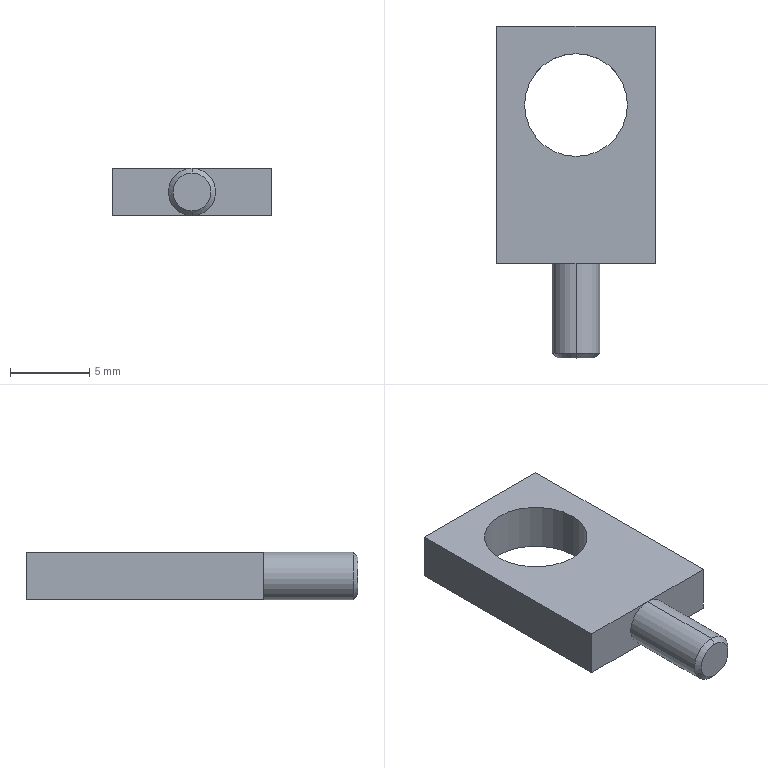Part | STEP file | 06-01-12 laser rotary plate | 1 solid | 14 faces | box 10 x 21 x 3 mm | volume 392.466 mm3 | plane 8 | cylinder 4 | cone 2 | commonest cylinder face diameters 3 x2 6.5 x2
STEP:
#1=CARTESIAN_POINT('',(0.,-13.5,0.3));
#2=VERTEX_POINT('',#1);
#3=CARTESIAN_POINT('',(0.,-13.5,2.7));
#4=VERTEX_POINT('',#3);
#5=CARTESIAN_POINT('',(0.,-13.5,1.5));
#6=DIRECTION('',(0.,-1.,0.));
#7=DIRECTION('',(0.,0.,-1.));
#8=AXIS2_PLACEMENT_3D('',#5,#6,#7);
#9=CIRCLE('',#8,1.2);
#10=EDGE_CURVE('',#2,#4,#9,.T.);
#11=ORIENTED_EDGE('',*,*,#10,.F.);
#12=CARTESIAN_POINT('',(0.,-13.2,0.));
#13=VERTEX_POINT('',#12);
#14=CARTESIAN_POINT('',(0.,-13.5,0.3));
#15=DIRECTION('',(0.,0.7071,-0.7071));
#16=VECTOR('',#15,1000.);
#17=LINE('',#14,#16);
#18=EDGE_CURVE('',#2,#13,#17,.T.);
#19=ORIENTED_EDGE('',*,*,#18,.T.);
#20=CARTESIAN_POINT('',(0.,-13.2,3.));
#21=VERTEX_POINT('',#20);
#22=CARTESIAN_POINT('',(0.,-13.2,1.5));
#23=DIRECTION('',(0.,1.,0.));
#24=DIRECTION('',(0.,0.,-1.));
#25=AXIS2_PLACEMENT_3D('',#22,#23,#24);
#26=CIRCLE('',#25,1.5);
#27=EDGE_CURVE('',#21,#13,#26,.T.);
#28=ORIENTED_EDGE('',*,*,#27,.F.);
#29=CARTESIAN_POINT('',(0.,-13.5,2.7));
#30=DIRECTION('',(0.,0.7071,0.7071));
#31=VECTOR('',#30,1000.);
#32=LINE('',#29,#31);
#33=EDGE_CURVE('',#4,#21,#32,.T.);
#34=ORIENTED_EDGE('',*,*,#33,.F.);
#35=EDGE_LOOP('',(#11,#19,#28,#34));
#36=FACE_OUTER_BOUND('',#35,.T.);
#37=CARTESIAN_POINT('',(0.,-13.5,1.5));
#38=DIRECTION('',(0.,1.,0.));
#39=DIRECTION('',(0.,0.,1.));
#40=AXIS2_PLACEMENT_3D('',#37,#38,#39);
#41=CONICAL_SURFACE('',#40,1.2,0.7854);
#42=ADVANCED_FACE('',(#36),#41,.T.);
#43=ORIENTED_EDGE('',*,*,#27,.T.);
#44=CARTESIAN_POINT('',(0.,-7.5,0.));
#45=VERTEX_POINT('',#44);
#46=CARTESIAN_POINT('',(0.,-13.5,0.));
#47=DIRECTION('',(0.,1.,0.));
#48=VECTOR('',#47,1000.);
#49=LINE('',#46,#48);
#50=EDGE_CURVE('',#13,#45,#49,.T.);
#51=ORIENTED_EDGE('',*,*,#50,.T.);
#52=CARTESIAN_POINT('',(0.,-7.5,3.));
#53=VERTEX_POINT('',#52);
#54=CARTESIAN_POINT('',(0.,-7.5,1.5));
#55=DIRECTION('',(0.,-1.,0.));
#56=DIRECTION('',(0.,0.,-1.));
#57=AXIS2_PLACEMENT_3D('',#54,#55,#56);
#58=CIRCLE('',#57,1.5);
#59=EDGE_CURVE('',#45,#53,#58,.T.);
#60=ORIENTED_EDGE('',*,*,#59,.T.);
#61=CARTESIAN_POINT('',(0.,-13.5,3.));
#62=DIRECTION('',(0.,1.,0.));
#63=VECTOR('',#62,1000.);
#64=LINE('',#61,#63);
#65=EDGE_CURVE('',#21,#53,#64,.T.);
#66=ORIENTED_EDGE('',*,*,#65,.F.);
#67=EDGE_LOOP('',(#43,#51,#60,#66));
#68=FACE_OUTER_BOUND('',#67,.T.);
#69=CARTESIAN_POINT('',(0.,-13.5,1.5));
#70=DIRECTION('',(0.,1.,0.));
#71=DIRECTION('',(0.,0.,1.));
#72=AXIS2_PLACEMENT_3D('',#69,#70,#71);
#73=CYLINDRICAL_SURFACE('',#72,1.5);
#74=ADVANCED_FACE('',(#68),#73,.T.);
#75=CARTESIAN_POINT('',(-3.25,2.5,3.));
#76=VERTEX_POINT('',#75);
#77=CARTESIAN_POINT('',(3.25,2.5,3.));
#78=VERTEX_POINT('',#77);
#79=CARTESIAN_POINT('',(0.,2.5,3.));
#80=DIRECTION('',(0.,0.,1.));
#81=DIRECTION('',(1.,0.,0.));
#82=AXIS2_PLACEMENT_3D('',#79,#80,#81);
#83=CIRCLE('',#82,3.25);
#84=EDGE_CURVE('',#76,#78,#83,.T.);
#85=ORIENTED_EDGE('',*,*,#84,.T.);
#86=CARTESIAN_POINT('',(3.25,2.5,0.));
#87=VERTEX_POINT('',#86);
#88=CARTESIAN_POINT('',(3.25,2.5,3.));
#89=DIRECTION('',(0.,0.,-1.));
#90=VECTOR('',#89,1000.);
#91=LINE('',#88,#90);
#92=EDGE_CURVE('',#78,#87,#91,.T.);
#93=ORIENTED_EDGE('',*,*,#92,.T.);
#94=CARTESIAN_POINT('',(-3.25,2.5,0.));
#95=VERTEX_POINT('',#94);
#96=CARTESIAN_POINT('',(0.,2.5,0.));
#97=DIRECTION('',(0.,0.,1.));
#98=DIRECTION('',(1.,0.,0.));
#99=AXIS2_PLACEMENT_3D('',#96,#97,#98);
#100=CIRCLE('',#99,3.25);
#101=EDGE_CURVE('',#95,#87,#100,.T.);
#102=ORIENTED_EDGE('',*,*,#101,.F.);
#103=CARTESIAN_POINT('',(-3.25,2.5,3.));
#104=DIRECTION('',(0.,0.,-1.));
#105=VECTOR('',#104,1000.);
#106=LINE('',#103,#105);
#107=EDGE_CURVE('',#76,#95,#106,.T.);
#108=ORIENTED_EDGE('',*,*,#107,.F.);
#109=EDGE_LOOP('',(#85,#93,#102,#108));
#110=FACE_OUTER_BOUND('',#109,.T.);
#111=CARTESIAN_POINT('',(0.,2.5,3.));
#112=DIRECTION('',(0.,0.,-1.));
#113=DIRECTION('',(-1.,0.,0.));
#114=AXIS2_PLACEMENT_3D('',#111,#112,#113);
#115=CYLINDRICAL_SURFACE('',#114,3.25);
#116=ADVANCED_FACE('',(#110),#115,.F.);
#117=ORIENTED_EDGE('',*,*,#59,.F.);
#118=CARTESIAN_POINT('',(5.,-7.5,0.));
#119=VERTEX_POINT('',#118);
#120=CARTESIAN_POINT('',(-5.,-7.5,0.));
#121=DIRECTION('',(1.,0.,0.));
#122=VECTOR('',#121,1000.);
#123=LINE('',#120,#122);
#124=EDGE_CURVE('',#45,#119,#123,.T.);
#125=ORIENTED_EDGE('',*,*,#124,.T.);
#126=CARTESIAN_POINT('',(5.,-7.5,3.));
#127=VERTEX_POINT('',#126);
#128=CARTESIAN_POINT('',(5.,-7.5,3.));
#129=DIRECTION('',(0.,0.,-1.));
#130=VECTOR('',#129,1000.);
#131=LINE('',#128,#130);
#132=EDGE_CURVE('',#127,#119,#131,.T.);
#133=ORIENTED_EDGE('',*,*,#132,.F.);
#134=CARTESIAN_POINT('',(-5.,-7.5,3.));
#135=DIRECTION('',(1.,0.,0.));
#136=VECTOR('',#135,1000.);
#137=LINE('',#134,#136);
#138=EDGE_CURVE('',#53,#127,#137,.T.);
#139=ORIENTED_EDGE('',*,*,#138,.F.);
#140=EDGE_LOOP('',(#117,#125,#133,#139));
#141=FACE_OUTER_BOUND('',#140,.T.);
#142=CARTESIAN_POINT('',(-5.,-7.5,3.));
#143=DIRECTION('',(0.,1.,0.));
#144=DIRECTION('',(0.,0.,1.));
#145=AXIS2_PLACEMENT_3D('',#142,#143,#144);
#146=PLANE('',#145);
#147=ADVANCED_FACE('',(#141),#146,.F.);
#148=CARTESIAN_POINT('',(0.,-7.5,1.5));
#149=DIRECTION('',(0.,-1.,0.));
#150=DIRECTION('',(0.,0.,-1.));
#151=AXIS2_PLACEMENT_3D('',#148,#149,#150);
#152=CIRCLE('',#151,1.5);
#153=EDGE_CURVE('',#53,#45,#152,.T.);
#154=ORIENTED_EDGE('',*,*,#153,.F.);
#155=CARTESIAN_POINT('',(-5.,-7.5,3.));
#156=VERTEX_POINT('',#155);
#157=CARTESIAN_POINT('',(-5.,-7.5,3.));
#158=DIRECTION('',(1.,0.,0.));
#159=VECTOR('',#158,1000.);
#160=LINE('',#157,#159);
#161=EDGE_CURVE('',#156,#53,#160,.T.);
#162=ORIENTED_EDGE('',*,*,#161,.F.);
#163=CARTESIAN_POINT('',(-5.,-7.5,0.));
#164=VERTEX_POINT('',#163);
#165=CARTESIAN_POINT('',(-5.,-7.5,3.));
#166=DIRECTION('',(0.,0.,-1.));
#167=VECTOR('',#166,1000.);
#168=LINE('',#165,#167);
#169=EDGE_CURVE('',#156,#164,#168,.T.);
#170=ORIENTED_EDGE('',*,*,#169,.T.);
#171=CARTESIAN_POINT('',(-5.,-7.5,0.));
#172=DIRECTION('',(1.,0.,0.));
#173=VECTOR('',#172,1000.);
#174=LINE('',#171,#173);
#175=EDGE_CURVE('',#164,#45,#174,.T.);
#176=ORIENTED_EDGE('',*,*,#175,.T.);
#177=EDGE_LOOP('',(#154,#162,#170,#176));
#178=FACE_OUTER_BOUND('',#177,.T.);
#179=CARTESIAN_POINT('',(-5.,-7.5,3.));
#180=DIRECTION('',(0.,1.,0.));
#181=DIRECTION('',(0.,0.,1.));
#182=AXIS2_PLACEMENT_3D('',#179,#180,#181);
#183=PLANE('',#182);
#184=ADVANCED_FACE('',(#178),#183,.F.);
#185=CARTESIAN_POINT('',(5.,7.5,3.));
#186=VERTEX_POINT('',#185);
#187=CARTESIAN_POINT('',(5.,7.5,3.));
#188=DIRECTION('',(0.,1.,0.));
#189=VECTOR('',#188,1000.);
#190=LINE('',#187,#189);
#191=EDGE_CURVE('',#127,#186,#190,.T.);
#192=ORIENTED_EDGE('',*,*,#191,.T.);
#193=CARTESIAN_POINT('',(-5.,7.5,3.));
#194=VERTEX_POINT('',#193);
#195=CARTESIAN_POINT('',(-5.,7.5,3.));
#196=DIRECTION('',(-1.,0.,0.));
#197=VECTOR('',#196,1000.);
#198=LINE('',#195,#197);
#199=EDGE_CURVE('',#186,#194,#198,.T.);
#200=ORIENTED_EDGE('',*,*,#199,.T.);
#201=CARTESIAN_POINT('',(-5.,7.5,3.));
#202=DIRECTION('',(0.,-1.,0.));
#203=VECTOR('',#202,1000.);
#204=LINE('',#201,#203);
#205=EDGE_CURVE('',#194,#156,#204,.T.);
#206=ORIENTED_EDGE('',*,*,#205,.T.);
#207=ORIENTED_EDGE('',*,*,#161,.T.);
#208=ORIENTED_EDGE('',*,*,#138,.T.);
#209=EDGE_LOOP('',(#192,#200,#206,#207,#208));
#210=FACE_OUTER_BOUND('',#209,.T.);
#211=ORIENTED_EDGE('',*,*,#84,.F.);
#212=CARTESIAN_POINT('',(0.,2.5,3.));
#213=DIRECTION('',(0.,0.,1.));
#214=DIRECTION('',(1.,0.,0.));
#215=AXIS2_PLACEMENT_3D('',#212,#213,#214);
#216=CIRCLE('',#215,3.25);
#217=EDGE_CURVE('',#78,#76,#216,.T.);
#218=ORIENTED_EDGE('',*,*,#217,.F.);
#219=EDGE_LOOP('',(#211,#218));
#220=FACE_BOUND('',#219,.T.);
#221=CARTESIAN_POINT('',(5.,-7.5,3.));
#222=DIRECTION('',(0.,0.,1.));
#223=DIRECTION('',(1.,0.,0.));
#224=AXIS2_PLACEMENT_3D('',#221,#222,#223);
#225=PLANE('',#224);
#226=ADVANCED_FACE('',(#210,#220),#225,.T.);
#227=CARTESIAN_POINT('',(5.,7.5,0.));
#228=VERTEX_POINT('',#227);
#229=CARTESIAN_POINT('',(5.,7.5,0.));
#230=DIRECTION('',(0.,1.,0.));
#231=VECTOR('',#230,1000.);
#232=LINE('',#229,#231);
#233=EDGE_CURVE('',#119,#228,#232,.T.);
#234=ORIENTED_EDGE('',*,*,#233,.F.);
#235=ORIENTED_EDGE('',*,*,#124,.F.);
#236=ORIENTED_EDGE('',*,*,#175,.F.);
#237=CARTESIAN_POINT('',(-5.,7.5,0.));
#238=VERTEX_POINT('',#237);
#239=CARTESIAN_POINT('',(-5.,7.5,0.));
#240=DIRECTION('',(0.,-1.,0.));
#241=VECTOR('',#240,1000.);
#242=LINE('',#239,#241);
#243=EDGE_CURVE('',#238,#164,#242,.T.);
#244=ORIENTED_EDGE('',*,*,#243,.F.);
#245=CARTESIAN_POINT('',(-5.,7.5,0.));
#246=DIRECTION('',(-1.,0.,0.));
#247=VECTOR('',#246,1000.);
#248=LINE('',#245,#247);
#249=EDGE_CURVE('',#228,#238,#248,.T.);
#250=ORIENTED_EDGE('',*,*,#249,.F.);
#251=EDGE_LOOP('',(#234,#235,#236,#244,#250));
#252=FACE_OUTER_BOUND('',#251,.T.);
#253=ORIENTED_EDGE('',*,*,#101,.T.);
#254=CARTESIAN_POINT('',(0.,2.5,0.));
#255=DIRECTION('',(0.,0.,1.));
#256=DIRECTION('',(1.,0.,0.));
#257=AXIS2_PLACEMENT_3D('',#254,#255,#256);
#258=CIRCLE('',#257,3.25);
#259=EDGE_CURVE('',#87,#95,#258,.T.);
#260=ORIENTED_EDGE('',*,*,#259,.T.);
#261=EDGE_LOOP('',(#253,#260));
#262=FACE_BOUND('',#261,.T.);
#263=CARTESIAN_POINT('',(5.,-7.5,0.));
#264=DIRECTION('',(0.,0.,1.));
#265=DIRECTION('',(1.,0.,0.));
#266=AXIS2_PLACEMENT_3D('',#263,#264,#265);
#267=PLANE('',#266);
#268=ADVANCED_FACE('',(#252,#262),#267,.F.);
#269=ORIENTED_EDGE('',*,*,#233,.T.);
#270=CARTESIAN_POINT('',(5.,7.5,3.));
#271=DIRECTION('',(0.,0.,-1.));
#272=VECTOR('',#271,1000.);
#273=LINE('',#270,#272);
#274=EDGE_CURVE('',#186,#228,#273,.T.);
#275=ORIENTED_EDGE('',*,*,#274,.F.);
#276=ORIENTED_EDGE('',*,*,#191,.F.);
#277=ORIENTED_EDGE('',*,*,#132,.T.);
#278=EDGE_LOOP('',(#269,#275,#276,#277));
#279=FACE_OUTER_BOUND('',#278,.T.);
#280=CARTESIAN_POINT('',(5.,7.5,3.));
#281=DIRECTION('',(-1.,0.,0.));
#282=DIRECTION('',(0.,-1.,0.));
#283=AXIS2_PLACEMENT_3D('',#280,#281,#282);
#284=PLANE('',#283);
#285=ADVANCED_FACE('',(#279),#284,.F.);
#286=ORIENTED_EDGE('',*,*,#249,.T.);
#287=CARTESIAN_POINT('',(-5.,7.5,3.));
#288=DIRECTION('',(0.,0.,-1.));
#289=VECTOR('',#288,1000.);
#290=LINE('',#287,#289);
#291=EDGE_CURVE('',#194,#238,#290,.T.);
#292=ORIENTED_EDGE('',*,*,#291,.F.);
#293=ORIENTED_EDGE('',*,*,#199,.F.);
#294=ORIENTED_EDGE('',*,*,#274,.T.);
#295=EDGE_LOOP('',(#286,#292,#293,#294));
#296=FACE_OUTER_BOUND('',#295,.T.);
#297=CARTESIAN_POINT('',(-5.,7.5,3.));
#298=DIRECTION('',(0.,-1.,0.));
#299=DIRECTION('',(0.,0.,-1.));
#300=AXIS2_PLACEMENT_3D('',#297,#298,#299);
#301=PLANE('',#300);
#302=ADVANCED_FACE('',(#296),#301,.F.);
#303=ORIENTED_EDGE('',*,*,#243,.T.);
#304=ORIENTED_EDGE('',*,*,#169,.F.);
#305=ORIENTED_EDGE('',*,*,#205,.F.);
#306=ORIENTED_EDGE('',*,*,#291,.T.);
#307=EDGE_LOOP('',(#303,#304,#305,#306));
#308=FACE_OUTER_BOUND('',#307,.T.);
#309=CARTESIAN_POINT('',(-5.,7.5,3.));
#310=DIRECTION('',(1.,0.,0.));
#311=DIRECTION('',(0.,1.,0.));
#312=AXIS2_PLACEMENT_3D('',#309,#310,#311);
#313=PLANE('',#312);
#314=ADVANCED_FACE('',(#308),#313,.F.);
#315=ORIENTED_EDGE('',*,*,#92,.F.);
#316=ORIENTED_EDGE('',*,*,#217,.T.);
#317=ORIENTED_EDGE('',*,*,#107,.T.);
#318=ORIENTED_EDGE('',*,*,#259,.F.);
#319=EDGE_LOOP('',(#315,#316,#317,#318));
#320=FACE_OUTER_BOUND('',#319,.T.);
#321=CARTESIAN_POINT('',(0.,2.5,3.));
#322=DIRECTION('',(0.,0.,-1.));
#323=DIRECTION('',(-1.,0.,0.));
#324=AXIS2_PLACEMENT_3D('',#321,#322,#323);
#325=CYLINDRICAL_SURFACE('',#324,3.25);
#326=ADVANCED_FACE('',(#320),#325,.F.);
#327=ORIENTED_EDGE('',*,*,#50,.F.);
#328=CARTESIAN_POINT('',(0.,-13.2,1.5));
#329=DIRECTION('',(0.,1.,0.));
#330=DIRECTION('',(0.,0.,-1.));
#331=AXIS2_PLACEMENT_3D('',#328,#329,#330);
#332=CIRCLE('',#331,1.5);
#333=EDGE_CURVE('',#13,#21,#332,.T.);
#334=ORIENTED_EDGE('',*,*,#333,.T.);
#335=ORIENTED_EDGE('',*,*,#65,.T.);
#336=ORIENTED_EDGE('',*,*,#153,.T.);
#337=EDGE_LOOP('',(#327,#334,#335,#336));
#338=FACE_OUTER_BOUND('',#337,.T.);
#339=CARTESIAN_POINT('',(0.,-13.5,1.5));
#340=DIRECTION('',(0.,1.,0.));
#341=DIRECTION('',(0.,0.,1.));
#342=AXIS2_PLACEMENT_3D('',#339,#340,#341);
#343=CYLINDRICAL_SURFACE('',#342,1.5);
#344=ADVANCED_FACE('',(#338),#343,.T.);
#345=CARTESIAN_POINT('',(0.,-13.5,1.5));
#346=DIRECTION('',(0.,-1.,0.));
#347=DIRECTION('',(0.,0.,-1.));
#348=AXIS2_PLACEMENT_3D('',#345,#346,#347);
#349=CIRCLE('',#348,1.2);
#350=EDGE_CURVE('',#4,#2,#349,.T.);
#351=ORIENTED_EDGE('',*,*,#350,.T.);
#352=ORIENTED_EDGE('',*,*,#10,.T.);
#353=EDGE_LOOP('',(#351,#352));
#354=FACE_OUTER_BOUND('',#353,.T.);
#355=CARTESIAN_POINT('',(0.,-13.5,1.5));
#356=DIRECTION('',(0.,-1.,0.));
#357=DIRECTION('',(0.,0.,-1.));
#358=AXIS2_PLACEMENT_3D('',#355,#356,#357);
#359=PLANE('',#358);
#360=ADVANCED_FACE('',(#354),#359,.T.);
#361=ORIENTED_EDGE('',*,*,#18,.F.);
#362=ORIENTED_EDGE('',*,*,#350,.F.);
#363=ORIENTED_EDGE('',*,*,#33,.T.);
#364=ORIENTED_EDGE('',*,*,#333,.F.);
#365=EDGE_LOOP('',(#361,#362,#363,#364));
#366=FACE_OUTER_BOUND('',#365,.T.);
#367=CARTESIAN_POINT('',(0.,-13.5,1.5));
#368=DIRECTION('',(0.,1.,0.));
#369=DIRECTION('',(0.,0.,1.));
#370=AXIS2_PLACEMENT_3D('',#367,#368,#369);
#371=CONICAL_SURFACE('',#370,1.2,0.7854);
#372=ADVANCED_FACE('',(#366),#371,.T.);
#373=CLOSED_SHELL('',(#42,#74,#116,#147,#184,#226,#268,#285,#302,#314,#326,#344,#360,#372));
#374=MANIFOLD_SOLID_BREP('',#373);
#375=CARTESIAN_POINT('',(0.,0.,0.));
#376=DIRECTION('',(0.,0.,1.));
#377=DIRECTION('',(1.,0.,0.));
#378=AXIS2_PLACEMENT_3D('',#375,#376,#377);
#379=(LENGTH_UNIT()NAMED_UNIT(*)SI_UNIT(.MILLI.,.METRE.));
#380=UNCERTAINTY_MEASURE_WITH_UNIT(LENGTH_MEASURE(0.00001),#379,'','');
#381=(NAMED_UNIT(*)PLANE_ANGLE_UNIT()SI_UNIT($,.RADIAN.));
#382=(NAMED_UNIT(*)SI_UNIT($,.STERADIAN.)SOLID_ANGLE_UNIT());
#383=(GEOMETRIC_REPRESENTATION_CONTEXT(3)GLOBAL_UNCERTAINTY_ASSIGNED_CONTEXT((#380))GLOBAL_UNIT_ASSIGNED_CONTEXT((#379,#381,#382))REPRESENTATION_CONTEXT('',''));
#384=ADVANCED_BREP_SHAPE_REPRESENTATION('',(#374,#378),#383);